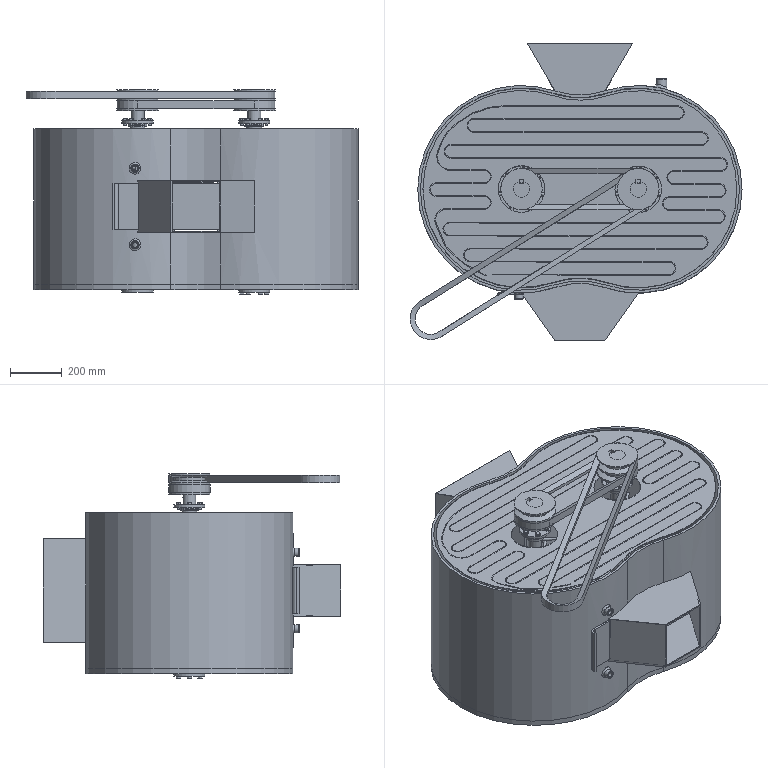Part | NX | 135 solids | 1010 faces | box 1280 x 1146 x 788 mm | volume 50655917 mm3 | plane 389 | cylinder 295 | cone 170 | torus 74 | sphere 72 | spline 10 | commonest cylinder face diameters 10 x70 3 x46 11 x24 9.732 x18 10.5 x18 18 x18